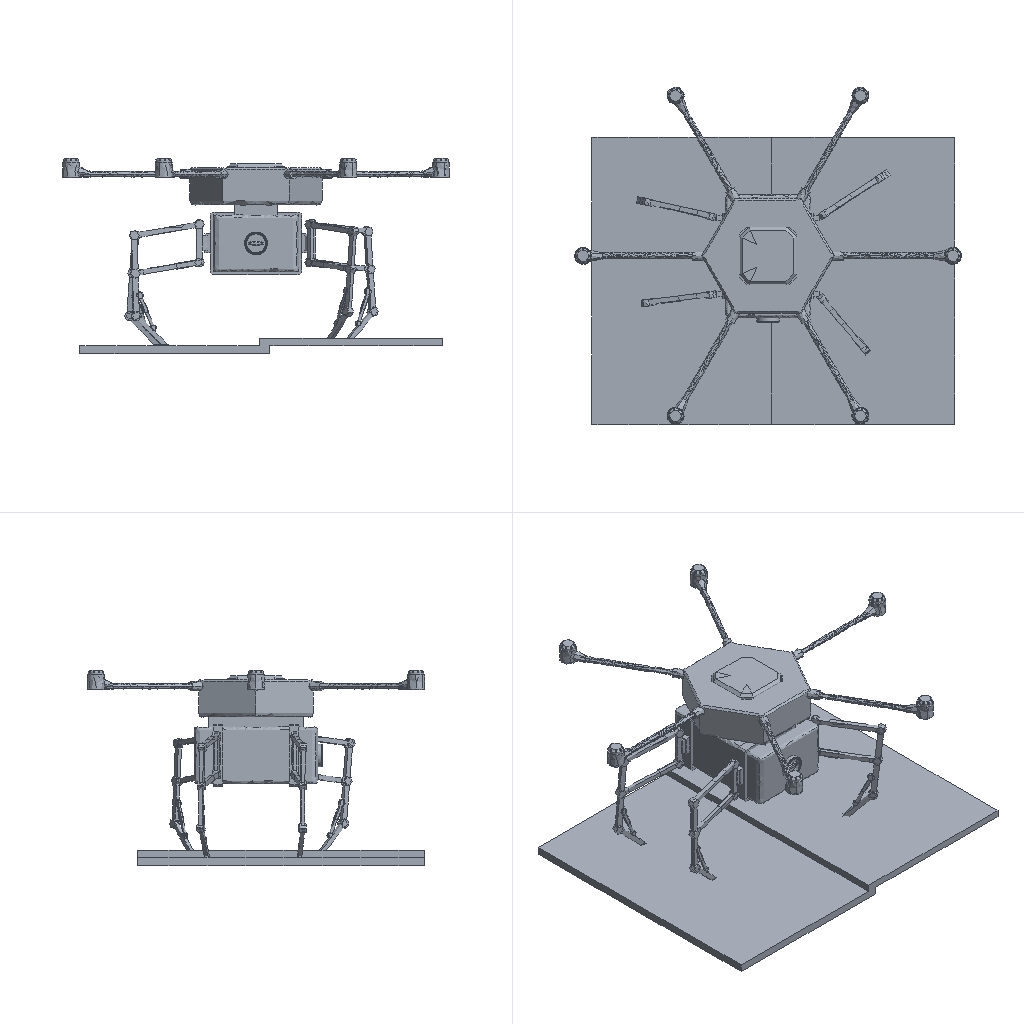Simulation study | ansys workbench
Ansys APDL input file, long lists of numbers shortened:
/batch
/config,noeldb,1     ! force off writing results to database
*get,_wallstrt,active,,time,wall
! ANSYS input file written by Workbench version 2022 R1
! File used for geometry attach:
/title,wbnew--____ (D5)
! ****** Begin Custom Load Command Snippet ******
/COM, ACT Extensions:
/COM,     LSDYNA, 2021.1
/COM,
! ****** End   Custom Load Command Snippet ******
*DIM,_wb_ProjectScratch_dir,string,248
_wb_ProjectScratch_dir(1) = ''
*DIM,_wb_SolverFiles_dir,string,248
_wb_SolverFiles_dir(1) = ''
*DIM,_wb_userfiles_dir,string,248
_wb_userfiles_dir(1) = ''
/com,--- Data in consistent NMM units. See Solving Units in the help system for more information.
/units,MPA
/nopr
/wb,file,start              !  signify a WB generated input file
/prep7
! Turn off shape checking because checks already performed inside WB mesher.
! See help system for more information.
SHPP,OFF,,NOWARN
/nolist
etcon,set             ! allow ANSYS to choose best KEYOP's for 180x elements, resets any applicable keyopt to MAPDL defaults
/com,*********** Nodes for the whole assembly ***********
nblock,3,,112600
(1i9,3e20.9e3)
        1    -5.098825787E+03     5.718523405E+02    -8.791296382E+02
! (102363 more lines like these left out)
-1
/wb,elem,start            !  set before creation of elements
/com,*********** Elements for Body 1 "xuanyi|dianjizhijia|Chamfer.1" ***********
et,1,187
eblock,19,solid,,480
(19i9)
        1        1        1        1        0        0        0        0       10        0     8464    14617    14621    14725    14652    14812    14839    14815    14813
! (959 more lines like these left out)
-1
/com,*********** Elements for Body 2 "xuanyi|jibi|Pad.1" ***********
et,2,187
eblock,19,solid,,1308
(19i9)
        2        2        2        2        0        0        0        0       10        0    42302    78362    78363    78430    78522    79436    79447    79438    79442
! (2615 more lines like these left out)
-1
/com,*********** Elements for Body 3 "xuanyi|xuanyidianji|CircPattern.1" ***********
et,3,187
eblock,19,solid,,3493
(19i9)
        3        3        3        3        0        0        0        0       10        0     9614    18655    18672    18754    18720    23347    23415    23351    23348
! (6985 more lines like these left out)
-1
/com,*********** Elements for Body 4 "xuanyi|dianjizhijia|Chamfer.1[2]" ***********
et,4,187
eblock,19,solid,,480
(19i9)
        4        4        4        4        0        0        0        0       10        0     7984    13609    13613    13717    13644    13804    13831    13807    13805
! (959 more lines like these left out)
-1
/com,*********** Elements for Body 5 "xuanyi|jibi|Pad.1[2]" ***********
et,5,187
eblock,19,solid,,1308
(19i9)
        5        5        5        5        0        0        0        0       10        0    39686    73092    73093    73160    73252    74166    74177    74168    74172
! (2615 more lines like these left out)
-1
! (50 more sections like these left out)
/wb,elem,end               !  done creating elements
/com,*********** Send User Defined Coordinate System(s) ***********
csys,0
toffst,273.15,  ! Temperature offset from absolute zero
/com,*********** Set Reference Temperature ***********
tref,22.
/wb,mat,start              !  starting to send materials
/com,*********** Send Materials ***********
Temperature = 'TEMP' ! Temperature
MP,DENS,1,7.85e-09,	! tonne mm^-3
MP,ALPX,1,1.2e-05,	! C^-1
MP,C,1,434000000,	! mm^2 s^-2 C^-1
MP,KXX,1,60.5,	! tonne mm s^-3 C^-1
MP,RSVX,1,0.00017,	! ohm mm
MP,EX,1,200000,	! tonne s^-2 mm^-1
MP,NUXY,1,0.3,
MP,MURX,1,10000,
Temperature = 'TEMP' ! Temperature
MP,DENS,2,7.85e-09,	! tonne mm^-3
MP,ALPX,2,1.2e-05,	! C^-1
MP,C,2,434000000,	! mm^2 s^-2 C^-1
MP,KXX,2,60.5,	! tonne mm s^-3 C^-1
MP,RSVX,2,0.00017,	! ohm mm
MP,EX,2,200000,	! tonne s^-2 mm^-1
MP,NUXY,2,0.3,
MP,MURX,2,10000,
Temperature = 'TEMP' ! Temperature
MP,DENS,3,7.85e-09,	! tonne mm^-3
MP,ALPX,3,1.2e-05,	! C^-1
MP,C,3,434000000,	! mm^2 s^-2 C^-1
MP,KXX,3,60.5,	! tonne mm s^-3 C^-1
MP,RSVX,3,0.00017,	! ohm mm
MP,EX,3,200000,	! tonne s^-2 mm^-1
MP,NUXY,3,0.3,
MP,MURX,3,10000,
Temperature = 'TEMP' ! Temperature
MP,DENS,4,7.85e-09,	! tonne mm^-3
MP,ALPX,4,1.2e-05,	! C^-1
MP,C,4,434000000,	! mm^2 s^-2 C^-1
MP,KXX,4,60.5,	! tonne mm s^-3 C^-1
MP,RSVX,4,0.00017,	! ohm mm
MP,EX,4,200000,	! tonne s^-2 mm^-1
MP,NUXY,4,0.3,
MP,MURX,4,10000,
Temperature = 'TEMP' ! Temperature
MP,DENS,5,7.85e-09,	! tonne mm^-3
MP,ALPX,5,1.2e-05,	! C^-1
MP,C,5,434000000,	! mm^2 s^-2 C^-1
MP,KXX,5,60.5,	! tonne mm s^-3 C^-1
MP,RSVX,5,0.00017,	! ohm mm
MP,EX,5,200000,	! tonne s^-2 mm^-1
MP,NUXY,5,0.3,
MP,MURX,5,10000,
Temperature = 'TEMP' ! Temperature
MP,DENS,6,7.85e-09,	! tonne mm^-3
MP,ALPX,6,1.2e-05,	! C^-1
MP,C,6,434000000,	! mm^2 s^-2 C^-1
MP,KXX,6,60.5,	! tonne mm s^-3 C^-1
MP,RSVX,6,0.00017,	! ohm mm
MP,EX,6,200000,	! tonne s^-2 mm^-1
MP,NUXY,6,0.3,
MP,MURX,6,10000,
Temperature = 'TEMP' ! Temperature
MP,DENS,7,7.85e-09,	! tonne mm^-3
MP,ALPX,7,1.2e-05,	! C^-1
MP,C,7,434000000,	! mm^2 s^-2 C^-1
MP,KXX,7,60.5,	! tonne mm s^-3 C^-1
MP,RSVX,7,0.00017,	! ohm mm
MP,EX,7,200000,	! tonne s^-2 mm^-1
MP,NUXY,7,0.3,
MP,MURX,7,10000,
Temperature = 'TEMP' ! Temperature
MP,DENS,8,7.85e-09,	! tonne mm^-3
MP,ALPX,8,1.2e-05,	! C^-1
MP,C,8,434000000,	! mm^2 s^-2 C^-1
MP,KXX,8,60.5,	! tonne mm s^-3 C^-1
MP,RSVX,8,0.00017,	! ohm mm
MP,EX,8,200000,	! tonne s^-2 mm^-1
MP,NUXY,8,0.3,
MP,MURX,8,10000,
Temperature = 'TEMP' ! Temperature
MP,DENS,9,7.85e-09,	! tonne mm^-3
MP,ALPX,9,1.2e-05,	! C^-1
MP,C,9,434000000,	! mm^2 s^-2 C^-1
MP,KXX,9,60.5,	! tonne mm s^-3 C^-1
MP,RSVX,9,0.00017,	! ohm mm
MP,EX,9,200000,	! tonne s^-2 mm^-1
! (416 more lines like these left out)
/wb,mat,end                !  done sending materials
!************************* Model Summary ********************
!xuanyi|dianjizhijia|Chamfer.1,	结构钢,	matid,	1
!xuanyi|jibi|Pad.1,	结构钢,	matid,	2
!xuanyi|xuanyidianji|CircPattern.1,	结构钢,	matid,	3
! (54 more lines like these left out)
*get,_xmin,node,,mnloc,x
*get,_ymin,node,,mnloc,y
*get,_zmin,node,,mnloc,z
*get,_xmax,node,,mxloc,x
*get,_ymax,node,,mxloc,y
*get,_zmax,node,,mxloc,z
_ASMDIAG=(_xmax-_xmin)*(_xmax-_xmin)+(_ymax-_ymin)*(_ymax-_ymin)+(_zmax-_zmin)*(_zmax-_zmin)
_ASMDIAG=SQRT(_ASMDIAG)
/wb,contact,start          !  starting to send contact
/com,*********** Create Contact "接触区域" ***********
/com,            Real Constant Set For Above Contact Is 57 & 56
*set,tid,57
*set,cid,56
r,tid
r,cid
et,tid,170
et,cid,174
eblock,10,,,60
(15i9)
    81102       57       57       57        0    14665    14758    14667    14667    15176    15196    14667    15170
! (59 more lines like these left out)
-1
eblock,10,,,60
(15i9)
    81162       56       56       56        0    14665    14758    14667    14667    15176    15196    14667    15170
! (59 more lines like these left out)
-1
eblock,10,,,74
(15i9)
    81222       56       57       56        0    78292    78299    78294    78294    78782    78791    78294    78780
! (73 more lines like these left out)
-1
eblock,10,,,74
(15i9)
    81296       57       56       57        0    78292    78299    78294    78294    78782    78791    78294    78780
! (73 more lines like these left out)
-1
keyo,cid,8,2               ! auto create asymmetric contact (from Program Controlled setting)
keyo,cid,10,0              ! adjust contact stiffness each NR iteration (from Program Controlled setting)
keyo,cid,12,5              ! bonded always
keyo,cid,18,1              ! small sliding turned on by application
keyo,cid,2,0               ! augmented Lagrange (from Program Controlled setting)
keyo,cid,4,0               ! on Gauss point (from Program Controlled setting)
keyo,cid,9,1               ! ignore initial gaps/penetration
keyo,cid,7,0               ! No Prediction
rmod,tid,3,10.      ! FKN
rmod,tid,5,0.       ! ICONT
rmod,tid,6,0.       ! PINB
rmod,tid,10,0.      ! CNOF
rmod,tid,12,0.      ! FKT
rmod,tid,36,230     ! WB DSID
rmod,cid,3,10.      ! FKN
rmod,cid,5,0.       ! ICONT
rmod,cid,6,0.       ! PINB
rmod,cid,10,0.      ! CNOF
rmod,cid,12,0.      ! FKT
rmod,cid,36,230     ! WB DSID
/com,*********** Create Contact "接触区域 2" ***********
/com,            Real Constant Set For Above Contact Is 59 & 58
*set,tid,59
*set,cid,58
r,tid
r,cid
et,tid,170
et,cid,174
eblock,10,,,78
(15i9)
    81370       59       59       59        0    14647    14649    14759    14759    15034    15054    14759    15039
! (77 more lines like these left out)
-1
eblock,10,,,78
(15i9)
    81448       58       58       58        0    14647    14649    14759    14759    15034    15054    14759    15039
! (77 more lines like these left out)
-1
eblock,10,,,254
(15i9)
    81526       58       59       58        0    18136    18346    18143    18143    20354    20406    18143    20350
! (253 more lines like these left out)
-1
eblock,10,,,254
(15i9)
    81780       59       58       59        0    18136    18346    18143    18143    20354    20406    18143    20350
! (253 more lines like these left out)
-1
keyo,cid,8,2               ! auto create asymmetric contact (from Program Controlled setting)
keyo,cid,10,0              ! adjust contact stiffness each NR iteration (from Program Controlled setting)
keyo,cid,12,5              ! bonded always
keyo,cid,18,1              ! small sliding turned on by application
keyo,cid,2,0               ! augmented Lagrange (from Program Controlled setting)
keyo,cid,4,0               ! on Gauss point (from Program Controlled setting)
keyo,cid,9,1               ! ignore initial gaps/penetration
keyo,cid,7,0               ! No Prediction
rmod,tid,3,10.      ! FKN
rmod,tid,5,0.       ! ICONT
rmod,tid,6,0.       ! PINB
rmod,tid,10,0.      ! CNOF
rmod,tid,12,0.      ! FKT
rmod,tid,36,233     ! WB DSID
rmod,cid,3,10.      ! FKN
rmod,cid,5,0.       ! ICONT
rmod,cid,6,0.       ! PINB
rmod,cid,10,0.      ! CNOF
rmod,cid,12,0.      ! FKT
rmod,cid,36,233     ! WB DSID
/com,*********** Create Contact "接触区域 3" ***********
/com,            Real Constant Set For Above Contact Is 61 & 60
*set,tid,61
*set,cid,60
r,tid
r,cid
et,tid,170
et,cid,174
eblock,10,,,85
(15i9)
    82034       61       61       61        0    78284    78291    78289    78289    78737    78766    78289    78736
! (84 more lines like these left out)
-1
eblock,10,,,85
(15i9)
    82119       60       60       60        0    78284    78291    78289    78289    78737    78766    78289    78736
! (84 more lines like these left out)
-1
eblock,10,,,62
(15i9)
    82204       60       61       60        0    47567    48345    47570    47570    52412    52438    47570    52410
! (61 more lines like these left out)
-1
eblock,10,,,62
(15i9)
    82266       61       60       61        0    47567    48345    47570    47570    52412    52438    47570    52410
! (61 more lines like these left out)
-1
keyo,cid,8,2               ! auto create asymmetric contact (from Program Controlled setting)
keyo,cid,10,0              ! adjust contact stiffness each NR iteration (from Program Controlled setting)
keyo,cid,12,5              ! bonded always
keyo,cid,18,1              ! small sliding turned on by application
keyo,cid,2,0               ! augmented Lagrange (from Program Controlled setting)
keyo,cid,4,0               ! on Gauss point (from Program Controlled setting)
keyo,cid,9,1               ! ignore initial gaps/penetration
keyo,cid,7,0               ! No Prediction
rmod,tid,3,10.      ! FKN
rmod,tid,5,0.       ! ICONT
rmod,tid,6,0.       ! PINB
rmod,tid,10,0.      ! CNOF
rmod,tid,12,0.      ! FKT
rmod,tid,36,236     ! WB DSID
rmod,cid,3,10.      ! FKN
rmod,cid,5,0.       ! ICONT
rmod,cid,6,0.       ! PINB
rmod,cid,10,0.      ! CNOF
rmod,cid,12,0.      ! FKT
rmod,cid,36,236     ! WB DSID
/com,*********** Create Contact "接触区域 8" ***********
/com,            Real Constant Set For Above Contact Is 63 & 62
*set,tid,63
*set,cid,62
r,tid
r,cid
et,tid,170
et,cid,174
eblock,10,,,60
(15i9)
    82328       63       63       63        0    13657    13750    13659    13659    14168    14188    13659    14162
! (59 more lines like these left out)
-1
eblock,10,,,60
(15i9)
    82388       62       62       62        0    13657    13750    13659    13659    14168    14188    13659    14162
! (59 more lines like these left out)
-1
eblock,10,,,74
(15i9)
    82448       62       63       62        0    73022    73029    73024    73024    73512    73521    73024    73510
! (73 more lines like these left out)
-1
eblock,10,,,74
(15i9)
    82522       63       62       63        0    73022    73029    73024    73024    73512    73521    73024    73510
! (73 more lines like these left out)
-1
keyo,cid,8,2               ! auto create asymmetric contact (from Program Controlled setting)
keyo,cid,10,0              ! adjust contact stiffness each NR iteration (from Program Controlled setting)
keyo,cid,12,5              ! bonded always
keyo,cid,18,1              ! small sliding turned on by application
keyo,cid,2,0               ! augmented Lagrange (from Program Controlled setting)
keyo,cid,4,0               ! on Gauss point (from Program Controlled setting)
keyo,cid,9,1               ! ignore initial gaps/penetration
keyo,cid,7,0               ! No Prediction
rmod,tid,3,10.      ! FKN
rmod,tid,5,0.       ! ICONT
rmod,tid,6,0.       ! PINB
rmod,tid,10,0.      ! CNOF
rmod,tid,12,0.      ! FKT
rmod,tid,36,251     ! WB DSID
rmod,cid,3,10.      ! FKN
rmod,cid,5,0.       ! ICONT
rmod,cid,6,0.       ! PINB
rmod,cid,10,0.      ! CNOF
rmod,cid,12,0.      ! FKT
rmod,cid,36,251     ! WB DSID
/com,*********** Create Contact "接触区域 9" ***********
/com,            Real Constant Set For Above Contact Is 65 & 64
*set,tid,65
*set,cid,64
r,tid
r,cid
et,tid,170
et,cid,174
eblock,10,,,78
(15i9)
    82596       65       65       65        0    13639    13641    13751    13751    14026    14046    13751    14031
! (77 more lines like these left out)
-1
eblock,10,,,78
(15i9)
    82674       64       64       64        0    13639    13641    13751    13751    14026    14046    13751    14031
! (77 more lines like these left out)
-1
eblock,10,,,254
(15i9)
    82752       64       65       64        0     8200     8410     8207     8207    10418    10470     8207    10414
! (253 more lines like these left out)
-1
eblock,10,,,254
(15i9)
    83006       65       64       65        0     8200     8410     8207     8207    10418    10470     8207    10414
! (253 more lines like these left out)
-1
keyo,cid,8,2               ! auto create asymmetric contact (from Program Controlled setting)
keyo,cid,10,0              ! adjust contact stiffness each NR iteration (from Program Controlled setting)
keyo,cid,12,5              ! bonded always
keyo,cid,18,1              ! small sliding turned on by application
keyo,cid,2,0               ! augmented Lagrange (from Program Controlled setting)
keyo,cid,4,0               ! on Gauss point (from Program Controlled setting)
keyo,cid,9,1               ! ignore initial gaps/penetration
keyo,cid,7,0               ! No Prediction
rmod,tid,3,10.      ! FKN
rmod,tid,5,0.       ! ICONT
rmod,tid,6,0.       ! PINB
rmod,tid,10,0.      ! CNOF
rmod,tid,12,0.      ! FKT
rmod,tid,36,254     ! WB DSID
rmod,cid,3,10.      ! FKN
rmod,cid,5,0.       ! ICONT
rmod,cid,6,0.       ! PINB
rmod,cid,10,0.      ! CNOF
rmod,cid,12,0.      ! FKT
rmod,cid,36,254     ! WB DSID
! (58 more sections like these left out)
/wb,contact,end            !  done creating contacts
/golist
/wb,load,start             !  starting to send loads
/com,*********** Fixed Supports ***********
CMBLOCK,_FIXEDSU,NODE,     6558
(8i10)
         1         3         5         6         7         8         9        10
! (819 more lines like these left out)
cmsel,s,_FIXEDSU
d,all,all
nsel,all
/com,*********** Define Force Using Surface Effect Elements ***********
local,12,0,0.,0.,0.,0.,0.,0.
csys,0
et,182,154
eblock,10,,,710
(15i9)
    93808      182      182      182       12    48190    48257    48280    48280    55610    56083    48280    55612
! (709 more lines like these left out)
-1
esel,s,type,,182
keyop,182,2,1                ! Apply load in local coordinate system
keyop,182,7,1                ! Use original area so load is constant in large deformation
esel,all
/gst,on,on
fini
*get,_numnode,node,0,count
*get,_numelem,elem,0,count
*get, _MAXELEMNUM, elem, 0, NUM, MAX
*get, _MAXNODENUM, node, 0, NUM, MAX
*get, _MAXELEMTYPE, etyp, 0, NUM, MAX
*get, _MAXREALCONST, real, 0, NUM, MAX
/go
/wb,load,end               !  done creating loads
/com,--- Number of total nodes = %_numnode%
/com,--- Number of contact elements = 13416
/com,--- Number of spring elements = 0
/com,--- Number of bearing elements = 0
/com,--- Number of solid elements = 55575
/com,--- Number of condensed parts = 0
/com,--- Number of total elements = %_numelem%
*get,_wallbsol,active,,time,wall
/com,****************************************************************************
/com,*************************    SOLUTION       ********************************
/com,****************************************************************************
/solu
antype,0                   ! static analysis
_thickRatio=0.164   ! Ratio of thick parts in the model
eqsl,sparse,,,,,1
cntr,print,1               ! print out contact info and also make no initial contact an error
dmpoption,emat,no             ! Don't combine emat file for DANSYS
dmpoption,esav,no             ! Don't combine esav file for DANSYS
nldiag,cont,iter           ! print out contact info each equilibrium iteration
rescontrol,,none                 ! Do not keep any restart files
/com,****************************************************
/com,******************* SOLVE FOR LS 1 OF 1 ****************
esel,s,type,,182
nsle
sfe,all,1,pres,1,0.
sfe,all,2,pres,1,0.
sfe,all,3,pres,1,-23.308
nsel,all
esel,all
/nopr
/gopr
nsub,1,1,1
time,1.
outres,erase
outres,all,none
outres,nsol,all,
outres,rsol,all
outres,eangl,all
outres,etmp,all
outres,veng,all
outres,strs,all,
outres,epel,all,
outres,eppl,all,
outres,cont,all,
! *********** WB SOLVE COMMAND ***********
! check interactive state
*get,ANSINTER_,active,,int
*if,ANSINTER_,ne,0,then
/eof
*endif
solve
/com *************** Write FE CONNECTORS *********
CEWRITE,file,ce,,INTE
/com,****************************************************
/com,*************** FINISHED SOLVE FOR LS 1 *************
*get,_wallasol,active,,time,wall
/nopr
*get,_numnode,node,0,count
*get,_numelem,elem,0,count
*get, _MAXELEMNUM, elem, 0, NUM, MAX
*get, _MAXNODENUM, node, 0, NUM, MAX,,,INTERNAL
*get, _MAXELEMTYPE, etyp, 0, NUM, MAX
*get, _MAXREALCONST, real, 0, NUM, MAX
/gopr
/post1
xmlo,ENCODING,ISO-8859-1
xmlo,parm
/xml,parm,xml
fini
/gopr
*get,_walldone,active,,time,wall
_preptime=(_wallbsol-_wallstrt)*3600
_solvtime=(_wallasol-_wallbsol)*3600
_posttime=(_walldone-_wallasol)*3600
_totaltim=(_walldone-_wallstrt)*3600
*get,_dlbratio,active,0,solu,dlbr
*get,_combtime,active,0,solu,comb
*get,_ssmode,active,0,solu,ssmm
*get,_ndofs,active,0,solu,ndof
*get,_sol_end_time,active,0,set,time
*if,_sol_end_time,eq,1.,then
/fclean				!clean distributed files
*endif
/com,--- Total number of nodes = %_numnode%
/com,--- Total number of elements = %_numelem%
/com,--- Element load balance ratio = %_dlbratio%
/com,--- Time to combine distributed files = %_combtime%
/com,--- Sparse memory mode = %_ssmode%
/com,--- Number of DOF = %_ndofs%
/wb,file,end               ! done with WB generated input